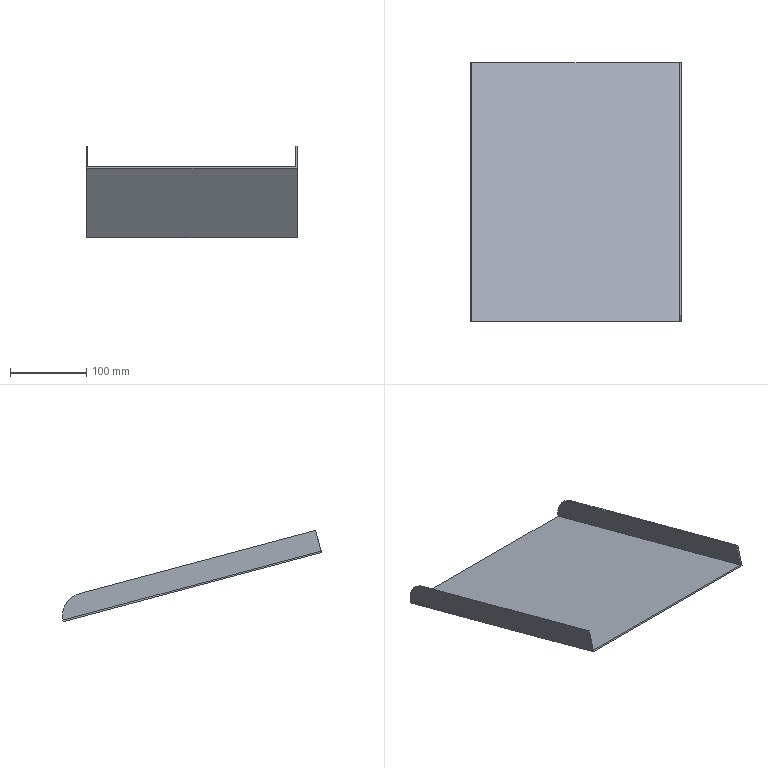Part | NX | features solid 2 | 1 solid | 12 faces | box 275.695 x 339.096 x 119.564 mm | volume 221807 mm3 | plane 10 | cylinder 2 | commonest cylinder face diameters 60 x2
STEP:
#1=CARTESIAN_POINT('',(556.256,1203.121,-600.755));
#2=VERTEX_POINT('',#1);
#3=CARTESIAN_POINT('',(557.256,1203.121,-600.755));
#4=VERTEX_POINT('',#3);
#5=CARTESIAN_POINT('',(556.256,1203.121,-600.755));
#6=CARTESIAN_POINT('',(556.59,1203.121,-600.755));
#7=CARTESIAN_POINT('',(556.923,1203.121,-600.755));
#8=CARTESIAN_POINT('',(557.256,1203.121,-600.755));
#9=B_SPLINE_CURVE_WITH_KNOTS('',3,(#5,#6,#7,#8),.UNSPECIFIED.,.F.,.F.,(4,4),(1310.709,1310.71),.UNSPECIFIED.);
#10=EDGE_CURVE('',#2,#4,#9,.T.);
#11=ORIENTED_EDGE('',*,*,#10,.T.);
#12=CARTESIAN_POINT('',(557.256,865.111,-510.186));
#13=VERTEX_POINT('',#12);
#14=CARTESIAN_POINT('',(557.256,1038.978,-556.773));
#15=DIRECTION('',(0.,-0.9659,0.2588));
#16=VECTOR('',#15,1000.);
#17=LINE('',#14,#16);
#18=EDGE_CURVE('',#4,#13,#17,.T.);
#19=ORIENTED_EDGE('',*,*,#18,.T.);
#20=CARTESIAN_POINT('',(829.951,865.111,-510.186));
#21=VERTEX_POINT('',#20);
#22=CARTESIAN_POINT('',(829.951,865.111,-510.186));
#23=DIRECTION('',(-1.,0.,0.));
#24=VECTOR('',#23,1000.);
#25=LINE('',#22,#24);
#26=EDGE_CURVE('',#21,#13,#25,.T.);
#27=ORIENTED_EDGE('',*,*,#26,.F.);
#28=CARTESIAN_POINT('',(829.951,1203.121,-600.755));
#29=VERTEX_POINT('',#28);
#30=CARTESIAN_POINT('',(829.951,1038.978,-556.773));
#31=DIRECTION('',(0.,-0.9659,0.2588));
#32=VECTOR('',#31,1000.);
#33=LINE('',#30,#32);
#34=EDGE_CURVE('',#29,#21,#33,.T.);
#35=ORIENTED_EDGE('',*,*,#34,.F.);
#36=CARTESIAN_POINT('',(831.951,1203.121,-600.755));
#37=VERTEX_POINT('',#36);
#38=CARTESIAN_POINT('',(829.951,1203.121,-600.755));
#39=CARTESIAN_POINT('',(830.618,1203.121,-600.755));
#40=CARTESIAN_POINT('',(831.285,1203.121,-600.755));
#41=CARTESIAN_POINT('',(831.951,1203.121,-600.755));
#42=B_SPLINE_CURVE_WITH_KNOTS('',3,(#38,#39,#40,#41),.UNSPECIFIED.,.F.,.F.,(4,4),(1310.689,1310.691),.UNSPECIFIED.);
#43=EDGE_CURVE('',#29,#37,#42,.T.);
#44=ORIENTED_EDGE('',*,*,#43,.T.);
#45=CARTESIAN_POINT('',(831.951,1203.185,-600.773));
#46=VERTEX_POINT('',#45);
#47=CARTESIAN_POINT('',(831.951,1038.978,-556.773));
#48=DIRECTION('',(0.,-0.9659,0.2588));
#49=VECTOR('',#48,1000.);
#50=LINE('',#47,#49);
#51=EDGE_CURVE('',#37,#46,#50,.F.);
#52=ORIENTED_EDGE('',*,*,#51,.T.);
#53=CARTESIAN_POINT('',(556.256,1203.185,-600.773));
#54=VERTEX_POINT('',#53);
#55=CARTESIAN_POINT('',(829.951,1203.185,-600.773));
#56=DIRECTION('',(-1.,0.,0.));
#57=VECTOR('',#56,1000.);
#58=LINE('',#55,#57);
#59=EDGE_CURVE('',#46,#54,#58,.T.);
#60=ORIENTED_EDGE('',*,*,#59,.T.);
#61=CARTESIAN_POINT('',(556.256,1038.978,-556.773));
#62=DIRECTION('',(0.,0.9659,-0.2588));
#63=VECTOR('',#62,1000.);
#64=LINE('',#61,#63);
#65=EDGE_CURVE('',#2,#54,#64,.T.);
#66=ORIENTED_EDGE('',*,*,#65,.F.);
#67=EDGE_LOOP('',(#11,#19,#27,#35,#44,#52,#60,#66));
#68=FACE_BOUND('',#67,.T.);
#69=CARTESIAN_POINT('',(829.951,1038.978,-556.773));
#70=DIRECTION('',(0.,-0.2588,-0.9659));
#71=DIRECTION('',(-1.,0.,0.));
#72=AXIS2_PLACEMENT_3D('',#69,#70,#71);
#73=PLANE('',#72);
#74=ADVANCED_FACE('',(#68),#73,.F.);
#75=ORIENTED_EDGE('',*,*,#26,.T.);
#76=CARTESIAN_POINT('',(557.256,872.358,-483.14));
#77=VERTEX_POINT('',#76);
#78=CARTESIAN_POINT('',(557.256,865.111,-510.186));
#79=DIRECTION('',(0.,0.2588,0.9659));
#80=VECTOR('',#79,1000.);
#81=LINE('',#78,#80);
#82=EDGE_CURVE('',#13,#77,#81,.T.);
#83=ORIENTED_EDGE('',*,*,#82,.T.);
#84=CARTESIAN_POINT('',(556.256,872.358,-483.14));
#85=VERTEX_POINT('',#84);
#86=CARTESIAN_POINT('',(546.256,872.358,-483.14));
#87=DIRECTION('',(-1.,0.,0.));
#88=VECTOR('',#87,1000.);
#89=LINE('',#86,#88);
#90=EDGE_CURVE('',#85,#77,#89,.F.);
#91=ORIENTED_EDGE('',*,*,#90,.F.);
#92=CARTESIAN_POINT('',(556.256,864.593,-512.118));
#93=VERTEX_POINT('',#92);
#94=CARTESIAN_POINT('',(556.256,865.111,-510.186));
#95=DIRECTION('',(0.,-0.2588,-0.9659));
#96=VECTOR('',#95,1000.);
#97=LINE('',#94,#96);
#98=EDGE_CURVE('',#85,#93,#97,.T.);
#99=ORIENTED_EDGE('',*,*,#98,.T.);
#100=CARTESIAN_POINT('',(831.951,864.593,-512.118));
#101=VERTEX_POINT('',#100);
#102=CARTESIAN_POINT('',(829.951,864.593,-512.118));
#103=DIRECTION('',(-1.,0.,0.));
#104=VECTOR('',#103,1000.);
#105=LINE('',#102,#104);
#106=EDGE_CURVE('',#101,#93,#105,.T.);
#107=ORIENTED_EDGE('',*,*,#106,.F.);
#108=CARTESIAN_POINT('',(831.951,872.358,-483.14));
#109=VERTEX_POINT('',#108);
#110=CARTESIAN_POINT('',(831.951,865.111,-510.186));
#111=DIRECTION('',(0.,0.2588,0.9659));
#112=VECTOR('',#111,1000.);
#113=LINE('',#110,#112);
#114=EDGE_CURVE('',#109,#101,#113,.F.);
#115=ORIENTED_EDGE('',*,*,#114,.F.);
#116=CARTESIAN_POINT('',(829.951,872.358,-483.14));
#117=VERTEX_POINT('',#116);
#118=CARTESIAN_POINT('',(841.951,872.358,-483.14));
#119=DIRECTION('',(-1.,0.,0.));
#120=VECTOR('',#119,1000.);
#121=LINE('',#118,#120);
#122=EDGE_CURVE('',#109,#117,#121,.T.);
#123=ORIENTED_EDGE('',*,*,#122,.T.);
#124=CARTESIAN_POINT('',(829.951,865.111,-510.186));
#125=DIRECTION('',(0.,0.2588,0.9659));
#126=VECTOR('',#125,1000.);
#127=LINE('',#124,#126);
#128=EDGE_CURVE('',#21,#117,#127,.T.);
#129=ORIENTED_EDGE('',*,*,#128,.F.);
#130=EDGE_LOOP('',(#75,#83,#91,#99,#107,#115,#123,#129));
#131=FACE_BOUND('',#130,.T.);
#132=CARTESIAN_POINT('',(829.951,865.111,-510.186));
#133=DIRECTION('',(0.,-0.9659,0.2588));
#134=DIRECTION('',(-1.,0.,0.));
#135=AXIS2_PLACEMENT_3D('',#132,#133,#134);
#136=PLANE('',#135);
#137=ADVANCED_FACE('',(#131),#136,.T.);
#138=CARTESIAN_POINT('',(556.256,1202.668,-602.704));
#139=VERTEX_POINT('',#138);
#140=CARTESIAN_POINT('',(556.256,1203.185,-600.773));
#141=DIRECTION('',(0.,0.2588,0.9659));
#142=VECTOR('',#141,1000.);
#143=LINE('',#140,#142);
#144=EDGE_CURVE('',#54,#139,#143,.F.);
#145=ORIENTED_EDGE('',*,*,#144,.T.);
#146=CARTESIAN_POINT('',(556.256,1038.46,-558.705));
#147=DIRECTION('',(0.,0.9659,-0.2588));
#148=VECTOR('',#147,1000.);
#149=LINE('',#146,#148);
#150=EDGE_CURVE('',#93,#139,#149,.T.);
#151=ORIENTED_EDGE('',*,*,#150,.F.);
#152=ORIENTED_EDGE('',*,*,#98,.F.);
#153=CARTESIAN_POINT('',(556.256,1181.454,-565.962));
#154=VERTEX_POINT('',#153);
#155=CARTESIAN_POINT('',(556.256,1046.225,-529.727));
#156=DIRECTION('',(0.,-0.9659,0.2588));
#157=VECTOR('',#156,1000.);
#158=LINE('',#155,#157);
#159=EDGE_CURVE('',#85,#154,#158,.F.);
#160=ORIENTED_EDGE('',*,*,#159,.T.);
#161=CARTESIAN_POINT('',(556.256,1173.69,-594.94));
#162=DIRECTION('',(-1.,0.,0.));
#163=DIRECTION('',(0.,0.,1.));
#164=AXIS2_PLACEMENT_3D('',#161,#162,#163);
#165=CIRCLE('',#164,30.);
#166=EDGE_CURVE('',#154,#2,#165,.T.);
#167=ORIENTED_EDGE('',*,*,#166,.T.);
#168=ORIENTED_EDGE('',*,*,#65,.T.);
#169=EDGE_LOOP('',(#145,#151,#152,#160,#167,#168));
#170=FACE_BOUND('',#169,.T.);
#171=CARTESIAN_POINT('',(556.256,1038.978,-556.773));
#172=DIRECTION('',(-1.,0.,0.));
#173=DIRECTION('',(0.,0.9659,-0.2588));
#174=AXIS2_PLACEMENT_3D('',#171,#172,#173);
#175=PLANE('',#174);
#176=ADVANCED_FACE('',(#170),#175,.T.);
#177=ORIENTED_EDGE('',*,*,#144,.F.);
#178=ORIENTED_EDGE('',*,*,#59,.F.);
#179=CARTESIAN_POINT('',(831.951,1202.668,-602.704));
#180=VERTEX_POINT('',#179);
#181=CARTESIAN_POINT('',(831.951,1203.185,-600.773));
#182=DIRECTION('',(0.,-0.2588,-0.9659));
#183=VECTOR('',#182,1000.);
#184=LINE('',#181,#183);
#185=EDGE_CURVE('',#46,#180,#184,.T.);
#186=ORIENTED_EDGE('',*,*,#185,.T.);
#187=CARTESIAN_POINT('',(829.951,1202.668,-602.704));
#188=DIRECTION('',(-1.,0.,0.));
#189=VECTOR('',#188,1000.);
#190=LINE('',#187,#189);
#191=EDGE_CURVE('',#180,#139,#190,.T.);
#192=ORIENTED_EDGE('',*,*,#191,.T.);
#193=EDGE_LOOP('',(#177,#178,#186,#192));
#194=FACE_BOUND('',#193,.T.);
#195=CARTESIAN_POINT('',(829.951,1203.185,-600.773));
#196=DIRECTION('',(0.,-0.9659,0.2588));
#197=DIRECTION('',(-1.,0.,0.));
#198=AXIS2_PLACEMENT_3D('',#195,#196,#197);
#199=PLANE('',#198);
#200=ADVANCED_FACE('',(#194),#199,.F.);
#201=ORIENTED_EDGE('',*,*,#106,.T.);
#202=ORIENTED_EDGE('',*,*,#150,.T.);
#203=ORIENTED_EDGE('',*,*,#191,.F.);
#204=CARTESIAN_POINT('',(831.951,1038.46,-558.705));
#205=DIRECTION('',(0.,-0.9659,0.2588));
#206=VECTOR('',#205,1000.);
#207=LINE('',#204,#206);
#208=EDGE_CURVE('',#101,#180,#207,.F.);
#209=ORIENTED_EDGE('',*,*,#208,.F.);
#210=EDGE_LOOP('',(#201,#202,#203,#209));
#211=FACE_BOUND('',#210,.T.);
#212=CARTESIAN_POINT('',(829.951,1038.46,-558.705));
#213=DIRECTION('',(0.,-0.2588,-0.9659));
#214=DIRECTION('',(-1.,0.,0.));
#215=AXIS2_PLACEMENT_3D('',#212,#213,#214);
#216=PLANE('',#215);
#217=ADVANCED_FACE('',(#211),#216,.T.);
#218=ORIENTED_EDGE('',*,*,#51,.F.);
#219=CARTESIAN_POINT('',(831.951,1181.454,-565.962));
#220=VERTEX_POINT('',#219);
#221=CARTESIAN_POINT('',(831.951,1173.69,-594.94));
#222=DIRECTION('',(-1.,0.,0.));
#223=DIRECTION('',(0.,0.,1.));
#224=AXIS2_PLACEMENT_3D('',#221,#222,#223);
#225=CIRCLE('',#224,30.);
#226=EDGE_CURVE('',#37,#220,#225,.F.);
#227=ORIENTED_EDGE('',*,*,#226,.T.);
#228=CARTESIAN_POINT('',(831.951,1046.225,-529.727));
#229=DIRECTION('',(0.,-0.9659,0.2588));
#230=VECTOR('',#229,1000.);
#231=LINE('',#228,#230);
#232=EDGE_CURVE('',#109,#220,#231,.F.);
#233=ORIENTED_EDGE('',*,*,#232,.F.);
#234=ORIENTED_EDGE('',*,*,#114,.T.);
#235=ORIENTED_EDGE('',*,*,#208,.T.);
#236=ORIENTED_EDGE('',*,*,#185,.F.);
#237=EDGE_LOOP('',(#218,#227,#233,#234,#235,#236));
#238=FACE_BOUND('',#237,.T.);
#239=CARTESIAN_POINT('',(831.951,1038.978,-556.773));
#240=DIRECTION('',(-1.,0.,0.));
#241=DIRECTION('',(0.,0.9659,-0.2588));
#242=AXIS2_PLACEMENT_3D('',#239,#240,#241);
#243=PLANE('',#242);
#244=ADVANCED_FACE('',(#238),#243,.F.);
#245=CARTESIAN_POINT('',(829.951,1181.454,-565.962));
#246=VERTEX_POINT('',#245);
#247=CARTESIAN_POINT('',(829.951,1173.69,-594.94));
#248=DIRECTION('',(1.,0.,0.));
#249=DIRECTION('',(0.,1.,0.));
#250=AXIS2_PLACEMENT_3D('',#247,#248,#249);
#251=CIRCLE('',#250,30.);
#252=EDGE_CURVE('',#246,#29,#251,.F.);
#253=ORIENTED_EDGE('',*,*,#252,.T.);
#254=ORIENTED_EDGE('',*,*,#34,.T.);
#255=ORIENTED_EDGE('',*,*,#128,.T.);
#256=CARTESIAN_POINT('',(829.951,1017.247,-521.963));
#257=DIRECTION('',(0.,0.9659,-0.2588));
#258=VECTOR('',#257,1000.);
#259=LINE('',#256,#258);
#260=EDGE_CURVE('',#117,#246,#259,.T.);
#261=ORIENTED_EDGE('',*,*,#260,.T.);
#262=EDGE_LOOP('',(#253,#254,#255,#261));
#263=FACE_BOUND('',#262,.T.);
#264=CARTESIAN_POINT('',(829.951,1009.482,-550.941));
#265=DIRECTION('',(1.,0.,0.));
#266=DIRECTION('',(0.,-0.2588,-0.9659));
#267=AXIS2_PLACEMENT_3D('',#264,#265,#266);
#268=PLANE('',#267);
#269=ADVANCED_FACE('',(#263),#268,.F.);
#270=ORIENTED_EDGE('',*,*,#43,.F.);
#271=ORIENTED_EDGE('',*,*,#252,.F.);
#272=CARTESIAN_POINT('',(841.951,1181.454,-565.962));
#273=DIRECTION('',(1.,0.,0.));
#274=VECTOR('',#273,1000.);
#275=LINE('',#272,#274);
#276=EDGE_CURVE('',#220,#246,#275,.F.);
#277=ORIENTED_EDGE('',*,*,#276,.F.);
#278=ORIENTED_EDGE('',*,*,#226,.F.);
#279=EDGE_LOOP('',(#270,#271,#277,#278));
#280=FACE_BOUND('',#279,.T.);
#281=CARTESIAN_POINT('',(841.951,1173.69,-594.94));
#282=DIRECTION('',(1.,0.,0.));
#283=DIRECTION('',(0.,-0.2588,-0.9659));
#284=AXIS2_PLACEMENT_3D('',#281,#282,#283);
#285=CYLINDRICAL_SURFACE('',#284,30.);
#286=ADVANCED_FACE('',(#280),#285,.T.);
#287=ORIENTED_EDGE('',*,*,#232,.T.);
#288=ORIENTED_EDGE('',*,*,#276,.T.);
#289=ORIENTED_EDGE('',*,*,#260,.F.);
#290=ORIENTED_EDGE('',*,*,#122,.F.);
#291=EDGE_LOOP('',(#287,#288,#289,#290));
#292=FACE_BOUND('',#291,.T.);
#293=CARTESIAN_POINT('',(841.951,1017.247,-521.963));
#294=DIRECTION('',(0.,-0.2588,-0.9659));
#295=DIRECTION('',(0.,0.9659,-0.2588));
#296=AXIS2_PLACEMENT_3D('',#293,#294,#295);
#297=PLANE('',#296);
#298=ADVANCED_FACE('',(#292),#297,.F.);
#299=ORIENTED_EDGE('',*,*,#18,.F.);
#300=CARTESIAN_POINT('',(557.256,1181.454,-565.962));
#301=VERTEX_POINT('',#300);
#302=CARTESIAN_POINT('',(557.256,1173.69,-594.94));
#303=DIRECTION('',(1.,0.,0.));
#304=DIRECTION('',(0.,1.,0.));
#305=AXIS2_PLACEMENT_3D('',#302,#303,#304);
#306=CIRCLE('',#305,30.);
#307=EDGE_CURVE('',#4,#301,#306,.T.);
#308=ORIENTED_EDGE('',*,*,#307,.T.);
#309=CARTESIAN_POINT('',(557.256,1017.247,-521.963));
#310=DIRECTION('',(0.,-0.9659,0.2588));
#311=VECTOR('',#310,1000.);
#312=LINE('',#309,#311);
#313=EDGE_CURVE('',#77,#301,#312,.F.);
#314=ORIENTED_EDGE('',*,*,#313,.F.);
#315=ORIENTED_EDGE('',*,*,#82,.F.);
#316=EDGE_LOOP('',(#299,#308,#314,#315));
#317=FACE_BOUND('',#316,.T.);
#318=CARTESIAN_POINT('',(557.256,1009.482,-550.941));
#319=DIRECTION('',(1.,0.,0.));
#320=DIRECTION('',(0.,-0.2588,-0.9659));
#321=AXIS2_PLACEMENT_3D('',#318,#319,#320);
#322=PLANE('',#321);
#323=ADVANCED_FACE('',(#317),#322,.T.);
#324=ORIENTED_EDGE('',*,*,#10,.F.);
#325=ORIENTED_EDGE('',*,*,#166,.F.);
#326=CARTESIAN_POINT('',(546.256,1181.454,-565.962));
#327=DIRECTION('',(1.,0.,0.));
#328=VECTOR('',#327,1000.);
#329=LINE('',#326,#328);
#330=EDGE_CURVE('',#301,#154,#329,.F.);
#331=ORIENTED_EDGE('',*,*,#330,.F.);
#332=ORIENTED_EDGE('',*,*,#307,.F.);
#333=EDGE_LOOP('',(#324,#325,#331,#332));
#334=FACE_BOUND('',#333,.T.);
#335=CARTESIAN_POINT('',(546.256,1173.69,-594.94));
#336=DIRECTION('',(-1.,0.,0.));
#337=DIRECTION('',(0.,0.2588,0.9659));
#338=AXIS2_PLACEMENT_3D('',#335,#336,#337);
#339=CYLINDRICAL_SURFACE('',#338,30.);
#340=ADVANCED_FACE('',(#334),#339,.T.);
#341=ORIENTED_EDGE('',*,*,#313,.T.);
#342=ORIENTED_EDGE('',*,*,#330,.T.);
#343=ORIENTED_EDGE('',*,*,#159,.F.);
#344=ORIENTED_EDGE('',*,*,#90,.T.);
#345=EDGE_LOOP('',(#341,#342,#343,#344));
#346=FACE_BOUND('',#345,.T.);
#347=CARTESIAN_POINT('',(546.256,1017.247,-521.963));
#348=DIRECTION('',(0.,-0.2588,-0.9659));
#349=DIRECTION('',(0.,0.9659,-0.2588));
#350=AXIS2_PLACEMENT_3D('',#347,#348,#349);
#351=PLANE('',#350);
#352=ADVANCED_FACE('',(#346),#351,.F.);
#353=CLOSED_SHELL('',(#74,#137,#176,#200,#217,#244,#269,#286,#298,#323,#340,#352));
#354=MANIFOLD_SOLID_BREP('',#353);
#355=(LENGTH_UNIT()NAMED_UNIT(*)SI_UNIT(.MILLI.,.METRE.));
#356=UNCERTAINTY_MEASURE_WITH_UNIT(LENGTH_MEASURE(0.0508),#355,'','');
#357=(NAMED_UNIT(*)PLANE_ANGLE_UNIT()SI_UNIT($,.RADIAN.));
#358=(NAMED_UNIT(*)SI_UNIT($,.STERADIAN.)SOLID_ANGLE_UNIT());
#359=(GEOMETRIC_REPRESENTATION_CONTEXT(3)GLOBAL_UNCERTAINTY_ASSIGNED_CONTEXT((#356))GLOBAL_UNIT_ASSIGNED_CONTEXT((#355,#357,#358))REPRESENTATION_CONTEXT('',''));
#360=ADVANCED_BREP_SHAPE_REPRESENTATION('',(#354),#359);